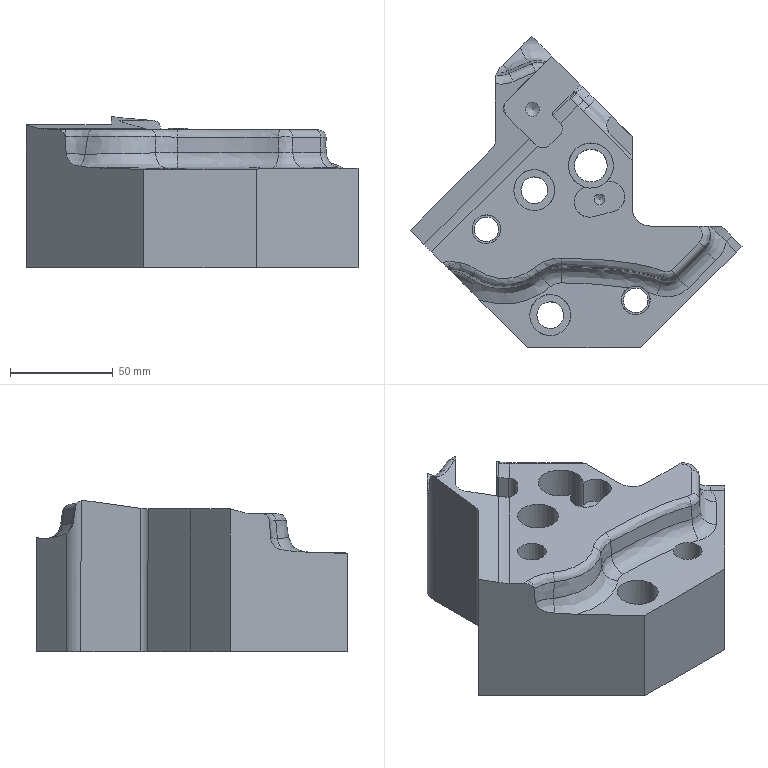Part | STEP file | gslz 2016.10.28-13_id526_x_t | 1 solid | 109 faces | box 161.927 x 152.068 x 73.808 mm | volume 667986 mm3 | spline 44 | plane 29 | cylinder 26 | other 8 | cone 2 | commonest cylinder face diameters 15 x4 12 x3 20 x3 7.5 x2 13 x2 14 x2